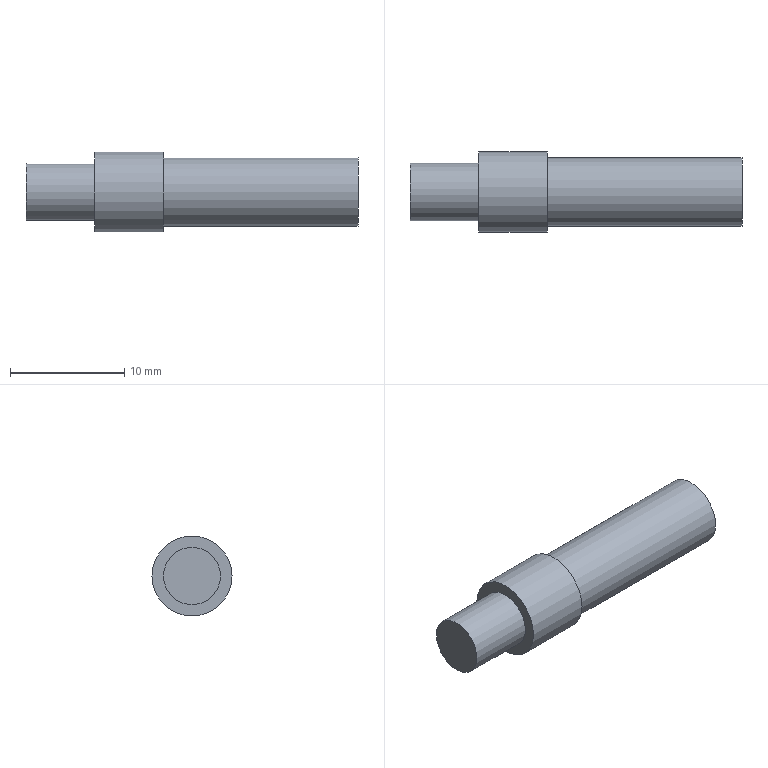Part | STEP file | 2-03.3 | 1 solid | 7 faces | box 29 x 7 x 7 mm | volume 829.38 mm3 | plane 4 | cylinder 3 | commonest cylinder face diameters 5 x1 6 x1 7 x1
STEP:
#1=CARTESIAN_POINT('',(0.,0.,0.));
#2=DIRECTION('',(0.,0.,1.));
#3=DIRECTION('',(1.,0.,0.));
#4=AXIS2_PLACEMENT_3D('',#1,#2,#3);
#5=CARTESIAN_POINT('',(0.,3.5,0.));
#6=VERTEX_POINT('',#5);
#7=CARTESIAN_POINT('',(-6.,3.5,0.));
#8=VERTEX_POINT('',#7);
#9=CARTESIAN_POINT('',(0.,3.5,0.));
#10=DIRECTION('',(-1.,0.,0.));
#11=VECTOR('',#10,1.);
#12=LINE('',#9,#11);
#13=CARTESIAN_POINT('',(0.,0.,0.));
#14=DIRECTION('',(-1.,0.,0.));
#15=DIRECTION('',(0.,1.,0.));
#16=AXIS2_PLACEMENT_3D('',#13,#14,#15);
#17=CYLINDRICAL_SURFACE('',#16,3.5);
#18=CARTESIAN_POINT('',(6.283,0.));
#19=DIRECTION('',(0.,1.));
#20=VECTOR('',#19,1.);
#21=LINE('',#18,#20);
#22=(GEOMETRIC_REPRESENTATION_CONTEXT(2)PARAMETRIC_REPRESENTATION_CONTEXT()REPRESENTATION_CONTEXT('',''));
#23=DEFINITIONAL_REPRESENTATION('',(#21),#22);
#24=PCURVE('',#17,#23);
#25=CARTESIAN_POINT('',(0.,0.));
#26=DIRECTION('',(0.,1.));
#27=VECTOR('',#26,1.);
#28=LINE('',#25,#27);
#29=(GEOMETRIC_REPRESENTATION_CONTEXT(2)PARAMETRIC_REPRESENTATION_CONTEXT()REPRESENTATION_CONTEXT('',''));
#30=DEFINITIONAL_REPRESENTATION('',(#28),#29);
#31=PCURVE('',#17,#30);
#32=SEAM_CURVE('',#12,(#24,#31),.PCURVE_S1.);
#33=EDGE_CURVE('',#6,#8,#32,.T.);
#34=ORIENTED_EDGE('',*,*,#33,.T.);
#35=CARTESIAN_POINT('',(-6.,0.,0.));
#36=DIRECTION('',(1.,0.,0.));
#37=DIRECTION('',(0.,1.,0.));
#38=AXIS2_PLACEMENT_3D('',#35,#36,#37);
#39=CIRCLE('',#38,3.5);
#40=CARTESIAN_POINT('',(6.283,6.));
#41=DIRECTION('',(-1.,0.));
#42=VECTOR('',#41,1.);
#43=LINE('',#40,#42);
#44=(GEOMETRIC_REPRESENTATION_CONTEXT(2)PARAMETRIC_REPRESENTATION_CONTEXT()REPRESENTATION_CONTEXT('',''));
#45=DEFINITIONAL_REPRESENTATION('',(#43),#44);
#46=PCURVE('',#17,#45);
#47=CARTESIAN_POINT('',(-6.,-0.9378,0.));
#48=DIRECTION('',(1.,0.,0.));
#49=DIRECTION('',(0.,0.,-1.));
#50=AXIS2_PLACEMENT_3D('',#47,#48,#49);
#51=PLANE('',#50);
#52=CARTESIAN_POINT('',(0.,0.9378));
#53=DIRECTION('',(0.,1.));
#54=AXIS2_PLACEMENT_2D('',#52,#53);
#55=CIRCLE('',#54,3.5);
#56=(GEOMETRIC_REPRESENTATION_CONTEXT(2)PARAMETRIC_REPRESENTATION_CONTEXT()REPRESENTATION_CONTEXT('',''));
#57=DEFINITIONAL_REPRESENTATION('',(#55),#56);
#58=PCURVE('',#51,#57);
#59=SURFACE_CURVE('',#39,(#46,#58),.PCURVE_S1.);
#60=EDGE_CURVE('',#8,#8,#59,.T.);
#61=ORIENTED_EDGE('',*,*,#60,.T.);
#62=ORIENTED_EDGE('',*,*,#33,.F.);
#63=CARTESIAN_POINT('',(0.,0.,0.));
#64=DIRECTION('',(1.,0.,0.));
#65=DIRECTION('',(0.,1.,0.));
#66=AXIS2_PLACEMENT_3D('',#63,#64,#65);
#67=CIRCLE('',#66,3.5);
#68=CARTESIAN_POINT('',(6.283,0.));
#69=DIRECTION('',(-1.,0.));
#70=VECTOR('',#69,1.);
#71=LINE('',#68,#70);
#72=(GEOMETRIC_REPRESENTATION_CONTEXT(2)PARAMETRIC_REPRESENTATION_CONTEXT()REPRESENTATION_CONTEXT('',''));
#73=DEFINITIONAL_REPRESENTATION('',(#71),#72);
#74=PCURVE('',#17,#73);
#75=CARTESIAN_POINT('',(0.,-0.9378,0.));
#76=DIRECTION('',(1.,0.,0.));
#77=DIRECTION('',(0.,0.,-1.));
#78=AXIS2_PLACEMENT_3D('',#75,#76,#77);
#79=PLANE('',#78);
#80=CARTESIAN_POINT('',(0.,0.9378));
#81=DIRECTION('',(0.,1.));
#82=AXIS2_PLACEMENT_2D('',#80,#81);
#83=CIRCLE('',#82,3.5);
#84=(GEOMETRIC_REPRESENTATION_CONTEXT(2)PARAMETRIC_REPRESENTATION_CONTEXT()REPRESENTATION_CONTEXT('',''));
#85=DEFINITIONAL_REPRESENTATION('',(#83),#84);
#86=PCURVE('',#79,#85);
#87=SURFACE_CURVE('',#67,(#74,#86),.PCURVE_S1.);
#88=EDGE_CURVE('',#6,#6,#87,.T.);
#89=ORIENTED_EDGE('',*,*,#88,.F.);
#90=EDGE_LOOP('',(#34,#61,#62,#89));
#91=FACE_BOUND('',#90,.T.);
#92=ADVANCED_FACE('',(#91),#17,.T.);
#93=ORIENTED_EDGE('',*,*,#88,.T.);
#94=EDGE_LOOP('',(#93));
#95=FACE_BOUND('',#94,.T.);
#96=CARTESIAN_POINT('',(0.,3.,0.));
#97=VERTEX_POINT('',#96);
#98=CARTESIAN_POINT('',(0.,0.,0.));
#99=DIRECTION('',(1.,0.,0.));
#100=DIRECTION('',(0.,1.,0.));
#101=AXIS2_PLACEMENT_3D('',#98,#99,#100);
#102=CIRCLE('',#101,3.);
#103=CARTESIAN_POINT('',(0.,0.9378));
#104=DIRECTION('',(0.,1.));
#105=AXIS2_PLACEMENT_2D('',#103,#104);
#106=CIRCLE('',#105,3.);
#107=(GEOMETRIC_REPRESENTATION_CONTEXT(2)PARAMETRIC_REPRESENTATION_CONTEXT()REPRESENTATION_CONTEXT('',''));
#108=DEFINITIONAL_REPRESENTATION('',(#106),#107);
#109=PCURVE('',#79,#108);
#110=CARTESIAN_POINT('',(0.,0.,0.));
#111=DIRECTION('',(1.,0.,0.));
#112=DIRECTION('',(0.,1.,0.));
#113=AXIS2_PLACEMENT_3D('',#110,#111,#112);
#114=CYLINDRICAL_SURFACE('',#113,3.);
#115=CARTESIAN_POINT('',(0.,0.));
#116=DIRECTION('',(1.,0.));
#117=VECTOR('',#116,1.);
#118=LINE('',#115,#117);
#119=(GEOMETRIC_REPRESENTATION_CONTEXT(2)PARAMETRIC_REPRESENTATION_CONTEXT()REPRESENTATION_CONTEXT('',''));
#120=DEFINITIONAL_REPRESENTATION('',(#118),#119);
#121=PCURVE('',#114,#120);
#122=SURFACE_CURVE('',#102,(#109,#121),.PCURVE_S1.);
#123=EDGE_CURVE('',#97,#97,#122,.T.);
#124=ORIENTED_EDGE('',*,*,#123,.F.);
#125=EDGE_LOOP('',(#124));
#126=FACE_BOUND('',#125,.T.);
#127=ADVANCED_FACE('',(#95,#126),#79,.T.);
#128=ORIENTED_EDGE('',*,*,#123,.T.);
#129=CARTESIAN_POINT('',(17.,3.,0.));
#130=VERTEX_POINT('',#129);
#131=CARTESIAN_POINT('',(0.,3.,0.));
#132=DIRECTION('',(1.,0.,0.));
#133=VECTOR('',#132,1.);
#134=LINE('',#131,#133);
#135=CARTESIAN_POINT('',(6.283,0.));
#136=DIRECTION('',(0.,1.));
#137=VECTOR('',#136,1.);
#138=LINE('',#135,#137);
#139=(GEOMETRIC_REPRESENTATION_CONTEXT(2)PARAMETRIC_REPRESENTATION_CONTEXT()REPRESENTATION_CONTEXT('',''));
#140=DEFINITIONAL_REPRESENTATION('',(#138),#139);
#141=PCURVE('',#114,#140);
#142=CARTESIAN_POINT('',(0.,0.));
#143=DIRECTION('',(0.,1.));
#144=VECTOR('',#143,1.);
#145=LINE('',#142,#144);
#146=(GEOMETRIC_REPRESENTATION_CONTEXT(2)PARAMETRIC_REPRESENTATION_CONTEXT()REPRESENTATION_CONTEXT('',''));
#147=DEFINITIONAL_REPRESENTATION('',(#145),#146);
#148=PCURVE('',#114,#147);
#149=SEAM_CURVE('',#134,(#141,#148),.PCURVE_S1.);
#150=EDGE_CURVE('',#97,#130,#149,.T.);
#151=ORIENTED_EDGE('',*,*,#150,.T.);
#152=CARTESIAN_POINT('',(17.,0.,0.));
#153=DIRECTION('',(1.,0.,0.));
#154=DIRECTION('',(0.,1.,0.));
#155=AXIS2_PLACEMENT_3D('',#152,#153,#154);
#156=CIRCLE('',#155,3.);
#157=CARTESIAN_POINT('',(0.,17.));
#158=DIRECTION('',(1.,0.));
#159=VECTOR('',#158,1.);
#160=LINE('',#157,#159);
#161=(GEOMETRIC_REPRESENTATION_CONTEXT(2)PARAMETRIC_REPRESENTATION_CONTEXT()REPRESENTATION_CONTEXT('',''));
#162=DEFINITIONAL_REPRESENTATION('',(#160),#161);
#163=PCURVE('',#114,#162);
#164=CARTESIAN_POINT('',(17.,-0.8038,0.));
#165=DIRECTION('',(1.,0.,0.));
#166=DIRECTION('',(0.,0.,-1.));
#167=AXIS2_PLACEMENT_3D('',#164,#165,#166);
#168=PLANE('',#167);
#169=CARTESIAN_POINT('',(0.,0.8038));
#170=DIRECTION('',(0.,1.));
#171=AXIS2_PLACEMENT_2D('',#169,#170);
#172=CIRCLE('',#171,3.);
#173=(GEOMETRIC_REPRESENTATION_CONTEXT(2)PARAMETRIC_REPRESENTATION_CONTEXT()REPRESENTATION_CONTEXT('',''));
#174=DEFINITIONAL_REPRESENTATION('',(#172),#173);
#175=PCURVE('',#168,#174);
#176=SURFACE_CURVE('',#156,(#163,#175),.PCURVE_S1.);
#177=EDGE_CURVE('',#130,#130,#176,.T.);
#178=ORIENTED_EDGE('',*,*,#177,.F.);
#179=ORIENTED_EDGE('',*,*,#150,.F.);
#180=EDGE_LOOP('',(#128,#151,#178,#179));
#181=FACE_BOUND('',#180,.T.);
#182=ADVANCED_FACE('',(#181),#114,.T.);
#183=ORIENTED_EDGE('',*,*,#177,.T.);
#184=EDGE_LOOP('',(#183));
#185=FACE_BOUND('',#184,.T.);
#186=ADVANCED_FACE('',(#185),#168,.T.);
#187=ORIENTED_EDGE('',*,*,#60,.T.);
#188=EDGE_LOOP('',(#187));
#189=FACE_BOUND('',#188,.F.);
#190=CARTESIAN_POINT('',(-6.,2.5,0.));
#191=VERTEX_POINT('',#190);
#192=CARTESIAN_POINT('',(-6.,0.,0.));
#193=DIRECTION('',(1.,0.,0.));
#194=DIRECTION('',(0.,1.,0.));
#195=AXIS2_PLACEMENT_3D('',#192,#193,#194);
#196=CIRCLE('',#195,2.5);
#197=CARTESIAN_POINT('',(0.,0.9378));
#198=DIRECTION('',(0.,1.));
#199=AXIS2_PLACEMENT_2D('',#197,#198);
#200=CIRCLE('',#199,2.5);
#201=(GEOMETRIC_REPRESENTATION_CONTEXT(2)PARAMETRIC_REPRESENTATION_CONTEXT()REPRESENTATION_CONTEXT('',''));
#202=DEFINITIONAL_REPRESENTATION('',(#200),#201);
#203=PCURVE('',#51,#202);
#204=CARTESIAN_POINT('',(-6.,0.,0.));
#205=DIRECTION('',(-1.,0.,0.));
#206=DIRECTION('',(0.,1.,0.));
#207=AXIS2_PLACEMENT_3D('',#204,#205,#206);
#208=CYLINDRICAL_SURFACE('',#207,2.5);
#209=CARTESIAN_POINT('',(6.283,0.));
#210=DIRECTION('',(-1.,0.));
#211=VECTOR('',#210,1.);
#212=LINE('',#209,#211);
#213=(GEOMETRIC_REPRESENTATION_CONTEXT(2)PARAMETRIC_REPRESENTATION_CONTEXT()REPRESENTATION_CONTEXT('',''));
#214=DEFINITIONAL_REPRESENTATION('',(#212),#213);
#215=PCURVE('',#208,#214);
#216=SURFACE_CURVE('',#196,(#203,#215),.PCURVE_S1.);
#217=EDGE_CURVE('',#191,#191,#216,.T.);
#218=ORIENTED_EDGE('',*,*,#217,.F.);
#219=EDGE_LOOP('',(#218));
#220=FACE_BOUND('',#219,.F.);
#221=ADVANCED_FACE('',(#189,#220),#51,.F.);
#222=CARTESIAN_POINT('',(-12.,2.5,0.));
#223=VERTEX_POINT('',#222);
#224=CARTESIAN_POINT('',(-6.,2.5,0.));
#225=DIRECTION('',(-1.,0.,0.));
#226=VECTOR('',#225,1.);
#227=LINE('',#224,#226);
#228=CARTESIAN_POINT('',(6.283,0.));
#229=DIRECTION('',(0.,1.));
#230=VECTOR('',#229,1.);
#231=LINE('',#228,#230);
#232=(GEOMETRIC_REPRESENTATION_CONTEXT(2)PARAMETRIC_REPRESENTATION_CONTEXT()REPRESENTATION_CONTEXT('',''));
#233=DEFINITIONAL_REPRESENTATION('',(#231),#232);
#234=PCURVE('',#208,#233);
#235=CARTESIAN_POINT('',(0.,0.));
#236=DIRECTION('',(0.,1.));
#237=VECTOR('',#236,1.);
#238=LINE('',#235,#237);
#239=(GEOMETRIC_REPRESENTATION_CONTEXT(2)PARAMETRIC_REPRESENTATION_CONTEXT()REPRESENTATION_CONTEXT('',''));
#240=DEFINITIONAL_REPRESENTATION('',(#238),#239);
#241=PCURVE('',#208,#240);
#242=SEAM_CURVE('',#227,(#234,#241),.PCURVE_S1.);
#243=EDGE_CURVE('',#191,#223,#242,.T.);
#244=ORIENTED_EDGE('',*,*,#243,.T.);
#245=CARTESIAN_POINT('',(-12.,0.,0.));
#246=DIRECTION('',(1.,0.,0.));
#247=DIRECTION('',(0.,1.,0.));
#248=AXIS2_PLACEMENT_3D('',#245,#246,#247);
#249=CIRCLE('',#248,2.5);
#250=CARTESIAN_POINT('',(6.283,6.));
#251=DIRECTION('',(-1.,0.));
#252=VECTOR('',#251,1.);
#253=LINE('',#250,#252);
#254=(GEOMETRIC_REPRESENTATION_CONTEXT(2)PARAMETRIC_REPRESENTATION_CONTEXT()REPRESENTATION_CONTEXT('',''));
#255=DEFINITIONAL_REPRESENTATION('',(#253),#254);
#256=PCURVE('',#208,#255);
#257=CARTESIAN_POINT('',(-12.,-0.6699,0.));
#258=DIRECTION('',(1.,0.,0.));
#259=DIRECTION('',(0.,0.,-1.));
#260=AXIS2_PLACEMENT_3D('',#257,#258,#259);
#261=PLANE('',#260);
#262=CARTESIAN_POINT('',(0.,0.6699));
#263=DIRECTION('',(0.,1.));
#264=AXIS2_PLACEMENT_2D('',#262,#263);
#265=CIRCLE('',#264,2.5);
#266=(GEOMETRIC_REPRESENTATION_CONTEXT(2)PARAMETRIC_REPRESENTATION_CONTEXT()REPRESENTATION_CONTEXT('',''));
#267=DEFINITIONAL_REPRESENTATION('',(#265),#266);
#268=PCURVE('',#261,#267);
#269=SURFACE_CURVE('',#249,(#256,#268),.PCURVE_S1.);
#270=EDGE_CURVE('',#223,#223,#269,.T.);
#271=ORIENTED_EDGE('',*,*,#270,.T.);
#272=ORIENTED_EDGE('',*,*,#243,.F.);
#273=ORIENTED_EDGE('',*,*,#217,.F.);
#274=EDGE_LOOP('',(#244,#271,#272,#273));
#275=FACE_BOUND('',#274,.T.);
#276=ADVANCED_FACE('',(#275),#208,.T.);
#277=ORIENTED_EDGE('',*,*,#270,.T.);
#278=EDGE_LOOP('',(#277));
#279=FACE_BOUND('',#278,.F.);
#280=ADVANCED_FACE('',(#279),#261,.F.);
#281=CLOSED_SHELL('',(#92,#127,#182,#186,#221,#276,#280));
#282=MANIFOLD_SOLID_BREP('',#281);
#283=(LENGTH_UNIT()NAMED_UNIT(*)SI_UNIT(.MILLI.,.METRE.));
#284=UNCERTAINTY_MEASURE_WITH_UNIT(LENGTH_MEASURE(0.0000001),#283,'','');
#285=(NAMED_UNIT(*)PLANE_ANGLE_UNIT()SI_UNIT($,.RADIAN.));
#286=(NAMED_UNIT(*)SI_UNIT($,.STERADIAN.)SOLID_ANGLE_UNIT());
#287=(GEOMETRIC_REPRESENTATION_CONTEXT(3)GLOBAL_UNCERTAINTY_ASSIGNED_CONTEXT((#284))GLOBAL_UNIT_ASSIGNED_CONTEXT((#283,#285,#286))REPRESENTATION_CONTEXT('',''));
#288=ADVANCED_BREP_SHAPE_REPRESENTATION('',(#4,#282),#287);